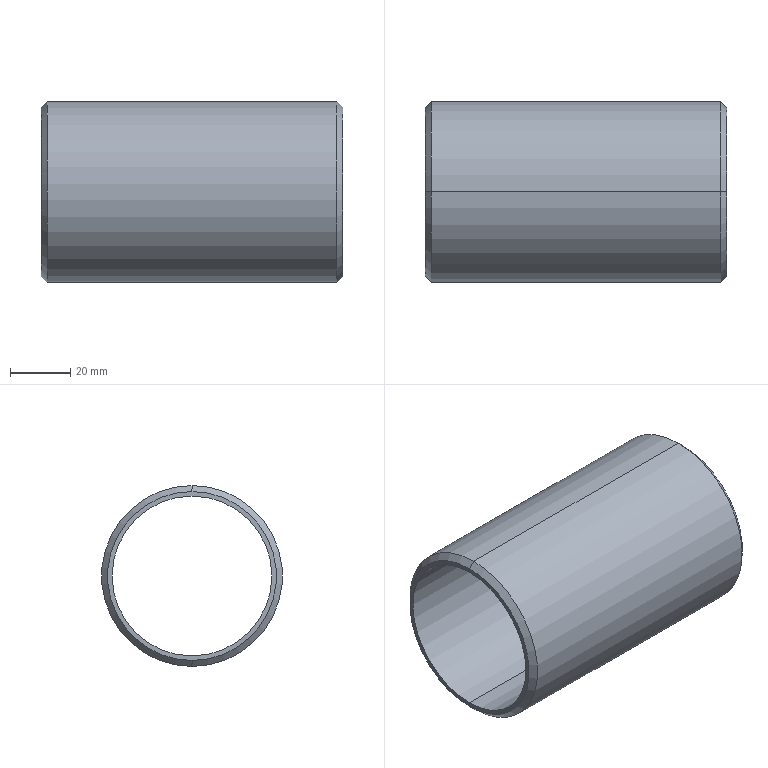Part | SolidWorks | features Chamfer 1, ExtruThin 1 | 1 solid | 10 faces | box 100 x 60 x 60 mm | volume 61388 mm3 | cone 4 | cylinder 4 | plane 2 | commonest cylinder face diameters 53 x2 60 x2
STEP:
#1=CARTESIAN_POINT('',(0.,0.,28.));
#2=VERTEX_POINT('',#1);
#3=CARTESIAN_POINT('',(0.,0.,-28.));
#4=VERTEX_POINT('',#3);
#5=CARTESIAN_POINT('',(0.,0.,0.));
#6=DIRECTION('',(-1.,0.,0.));
#7=DIRECTION('',(0.,0.,-1.));
#8=AXIS2_PLACEMENT_3D('',#5,#6,#7);
#9=CIRCLE('',#8,28.);
#10=EDGE_CURVE('',#2,#4,#9,.T.);
#11=ORIENTED_EDGE('',*,*,#10,.F.);
#12=CARTESIAN_POINT('',(2.,0.,30.));
#13=VERTEX_POINT('',#12);
#14=CARTESIAN_POINT('',(2.,0.,30.));
#15=DIRECTION('',(0.7071,0.,0.7071));
#16=VECTOR('',#15,1000.);
#17=LINE('',#14,#16);
#18=EDGE_CURVE('',#2,#13,#17,.T.);
#19=ORIENTED_EDGE('',*,*,#18,.T.);
#20=CARTESIAN_POINT('',(2.,0.,-30.));
#21=VERTEX_POINT('',#20);
#22=CARTESIAN_POINT('',(2.,0.,0.));
#23=DIRECTION('',(1.,0.,0.));
#24=DIRECTION('',(0.,0.,-1.));
#25=AXIS2_PLACEMENT_3D('',#22,#23,#24);
#26=CIRCLE('',#25,30.);
#27=EDGE_CURVE('',#21,#13,#26,.T.);
#28=ORIENTED_EDGE('',*,*,#27,.F.);
#29=CARTESIAN_POINT('',(2.,0.,-30.));
#30=DIRECTION('',(0.7071,0.,-0.7071));
#31=VECTOR('',#30,1000.);
#32=LINE('',#29,#31);
#33=EDGE_CURVE('',#4,#21,#32,.T.);
#34=ORIENTED_EDGE('',*,*,#33,.F.);
#35=EDGE_LOOP('',(#11,#19,#28,#34));
#36=FACE_OUTER_BOUND('',#35,.T.);
#37=CARTESIAN_POINT('',(2.,0.,0.));
#38=DIRECTION('',(1.,0.,0.));
#39=DIRECTION('',(0.,0.,-1.));
#40=AXIS2_PLACEMENT_3D('',#37,#38,#39);
#41=CONICAL_SURFACE('',#40,30.,0.7854);
#42=ADVANCED_FACE('',(#36),#41,.T.);
#43=CARTESIAN_POINT('',(100.,0.,-28.));
#44=VERTEX_POINT('',#43);
#45=CARTESIAN_POINT('',(100.,0.,28.));
#46=VERTEX_POINT('',#45);
#47=CARTESIAN_POINT('',(100.,0.,0.));
#48=DIRECTION('',(1.,0.,0.));
#49=DIRECTION('',(0.,0.,-1.));
#50=AXIS2_PLACEMENT_3D('',#47,#48,#49);
#51=CIRCLE('',#50,28.);
#52=EDGE_CURVE('',#44,#46,#51,.T.);
#53=ORIENTED_EDGE('',*,*,#52,.F.);
#54=CARTESIAN_POINT('',(98.,0.,-30.));
#55=VERTEX_POINT('',#54);
#56=CARTESIAN_POINT('',(100.,0.,-28.));
#57=DIRECTION('',(-0.7071,0.,-0.7071));
#58=VECTOR('',#57,1000.);
#59=LINE('',#56,#58);
#60=EDGE_CURVE('',#44,#55,#59,.T.);
#61=ORIENTED_EDGE('',*,*,#60,.T.);
#62=CARTESIAN_POINT('',(98.,0.,30.));
#63=VERTEX_POINT('',#62);
#64=CARTESIAN_POINT('',(98.,0.,0.));
#65=DIRECTION('',(-1.,0.,0.));
#66=DIRECTION('',(0.,0.,-1.));
#67=AXIS2_PLACEMENT_3D('',#64,#65,#66);
#68=CIRCLE('',#67,30.);
#69=EDGE_CURVE('',#63,#55,#68,.T.);
#70=ORIENTED_EDGE('',*,*,#69,.F.);
#71=CARTESIAN_POINT('',(100.,0.,28.));
#72=DIRECTION('',(-0.7071,0.,0.7071));
#73=VECTOR('',#72,1000.);
#74=LINE('',#71,#73);
#75=EDGE_CURVE('',#46,#63,#74,.T.);
#76=ORIENTED_EDGE('',*,*,#75,.F.);
#77=EDGE_LOOP('',(#53,#61,#70,#76));
#78=FACE_OUTER_BOUND('',#77,.T.);
#79=CARTESIAN_POINT('',(100.,0.,0.));
#80=DIRECTION('',(-1.,0.,0.));
#81=DIRECTION('',(0.,0.,1.));
#82=AXIS2_PLACEMENT_3D('',#79,#80,#81);
#83=CONICAL_SURFACE('',#82,28.,0.7854);
#84=ADVANCED_FACE('',(#78),#83,.T.);
#85=CARTESIAN_POINT('',(100.,0.,26.5));
#86=VERTEX_POINT('',#85);
#87=CARTESIAN_POINT('',(100.,0.,-26.5));
#88=VERTEX_POINT('',#87);
#89=CARTESIAN_POINT('',(100.,0.,0.));
#90=DIRECTION('',(1.,0.,0.));
#91=DIRECTION('',(0.,0.,-1.));
#92=AXIS2_PLACEMENT_3D('',#89,#90,#91);
#93=CIRCLE('',#92,26.5);
#94=EDGE_CURVE('',#86,#88,#93,.T.);
#95=ORIENTED_EDGE('',*,*,#94,.T.);
#96=CARTESIAN_POINT('',(0.,0.,-26.5));
#97=VERTEX_POINT('',#96);
#98=CARTESIAN_POINT('',(100.,0.,-26.5));
#99=DIRECTION('',(-1.,0.,0.));
#100=VECTOR('',#99,1000.);
#101=LINE('',#98,#100);
#102=EDGE_CURVE('',#88,#97,#101,.T.);
#103=ORIENTED_EDGE('',*,*,#102,.T.);
#104=CARTESIAN_POINT('',(0.,0.,26.5));
#105=VERTEX_POINT('',#104);
#106=CARTESIAN_POINT('',(0.,0.,0.));
#107=DIRECTION('',(1.,0.,0.));
#108=DIRECTION('',(0.,0.,-1.));
#109=AXIS2_PLACEMENT_3D('',#106,#107,#108);
#110=CIRCLE('',#109,26.5);
#111=EDGE_CURVE('',#105,#97,#110,.T.);
#112=ORIENTED_EDGE('',*,*,#111,.F.);
#113=CARTESIAN_POINT('',(100.,0.,26.5));
#114=DIRECTION('',(-1.,0.,0.));
#115=VECTOR('',#114,1000.);
#116=LINE('',#113,#115);
#117=EDGE_CURVE('',#86,#105,#116,.T.);
#118=ORIENTED_EDGE('',*,*,#117,.F.);
#119=EDGE_LOOP('',(#95,#103,#112,#118));
#120=FACE_OUTER_BOUND('',#119,.T.);
#121=CARTESIAN_POINT('',(100.,0.,0.));
#122=DIRECTION('',(-1.,0.,0.));
#123=DIRECTION('',(0.,0.,1.));
#124=AXIS2_PLACEMENT_3D('',#121,#122,#123);
#125=CYLINDRICAL_SURFACE('',#124,26.5);
#126=ADVANCED_FACE('',(#120),#125,.F.);
#127=ORIENTED_EDGE('',*,*,#69,.T.);
#128=CARTESIAN_POINT('',(100.,0.,-30.));
#129=DIRECTION('',(-1.,0.,0.));
#130=VECTOR('',#129,1000.);
#131=LINE('',#128,#130);
#132=EDGE_CURVE('',#55,#21,#131,.T.);
#133=ORIENTED_EDGE('',*,*,#132,.T.);
#134=ORIENTED_EDGE('',*,*,#27,.T.);
#135=CARTESIAN_POINT('',(100.,0.,30.));
#136=DIRECTION('',(-1.,0.,0.));
#137=VECTOR('',#136,1000.);
#138=LINE('',#135,#137);
#139=EDGE_CURVE('',#63,#13,#138,.T.);
#140=ORIENTED_EDGE('',*,*,#139,.F.);
#141=EDGE_LOOP('',(#127,#133,#134,#140));
#142=FACE_OUTER_BOUND('',#141,.T.);
#143=CARTESIAN_POINT('',(100.,0.,0.));
#144=DIRECTION('',(-1.,0.,0.));
#145=DIRECTION('',(0.,0.,1.));
#146=AXIS2_PLACEMENT_3D('',#143,#144,#145);
#147=CYLINDRICAL_SURFACE('',#146,30.);
#148=ADVANCED_FACE('',(#142),#147,.T.);
#149=CARTESIAN_POINT('',(100.,0.,0.));
#150=DIRECTION('',(1.,0.,0.));
#151=DIRECTION('',(0.,0.,-1.));
#152=AXIS2_PLACEMENT_3D('',#149,#150,#151);
#153=CIRCLE('',#152,28.);
#154=EDGE_CURVE('',#46,#44,#153,.T.);
#155=ORIENTED_EDGE('',*,*,#154,.T.);
#156=ORIENTED_EDGE('',*,*,#52,.T.);
#157=EDGE_LOOP('',(#155,#156));
#158=FACE_OUTER_BOUND('',#157,.T.);
#159=ORIENTED_EDGE('',*,*,#94,.F.);
#160=CARTESIAN_POINT('',(100.,0.,0.));
#161=DIRECTION('',(1.,0.,0.));
#162=DIRECTION('',(0.,0.,-1.));
#163=AXIS2_PLACEMENT_3D('',#160,#161,#162);
#164=CIRCLE('',#163,26.5);
#165=EDGE_CURVE('',#88,#86,#164,.T.);
#166=ORIENTED_EDGE('',*,*,#165,.F.);
#167=EDGE_LOOP('',(#159,#166));
#168=FACE_BOUND('',#167,.T.);
#169=CARTESIAN_POINT('',(100.,0.,0.));
#170=DIRECTION('',(1.,0.,0.));
#171=DIRECTION('',(0.,0.,-1.));
#172=AXIS2_PLACEMENT_3D('',#169,#170,#171);
#173=PLANE('',#172);
#174=ADVANCED_FACE('',(#158,#168),#173,.T.);
#175=CARTESIAN_POINT('',(0.,0.,0.));
#176=DIRECTION('',(-1.,0.,0.));
#177=DIRECTION('',(0.,0.,-1.));
#178=AXIS2_PLACEMENT_3D('',#175,#176,#177);
#179=CIRCLE('',#178,28.);
#180=EDGE_CURVE('',#4,#2,#179,.T.);
#181=ORIENTED_EDGE('',*,*,#180,.T.);
#182=ORIENTED_EDGE('',*,*,#10,.T.);
#183=EDGE_LOOP('',(#181,#182));
#184=FACE_OUTER_BOUND('',#183,.T.);
#185=ORIENTED_EDGE('',*,*,#111,.T.);
#186=CARTESIAN_POINT('',(0.,0.,0.));
#187=DIRECTION('',(1.,0.,0.));
#188=DIRECTION('',(0.,0.,-1.));
#189=AXIS2_PLACEMENT_3D('',#186,#187,#188);
#190=CIRCLE('',#189,26.5);
#191=EDGE_CURVE('',#97,#105,#190,.T.);
#192=ORIENTED_EDGE('',*,*,#191,.T.);
#193=EDGE_LOOP('',(#185,#192));
#194=FACE_BOUND('',#193,.T.);
#195=CARTESIAN_POINT('',(0.,0.,0.));
#196=DIRECTION('',(1.,0.,0.));
#197=DIRECTION('',(0.,0.,-1.));
#198=AXIS2_PLACEMENT_3D('',#195,#196,#197);
#199=PLANE('',#198);
#200=ADVANCED_FACE('',(#184,#194),#199,.F.);
#201=ORIENTED_EDGE('',*,*,#132,.F.);
#202=CARTESIAN_POINT('',(98.,0.,0.));
#203=DIRECTION('',(-1.,0.,0.));
#204=DIRECTION('',(0.,0.,-1.));
#205=AXIS2_PLACEMENT_3D('',#202,#203,#204);
#206=CIRCLE('',#205,30.);
#207=EDGE_CURVE('',#55,#63,#206,.T.);
#208=ORIENTED_EDGE('',*,*,#207,.T.);
#209=ORIENTED_EDGE('',*,*,#139,.T.);
#210=CARTESIAN_POINT('',(2.,0.,0.));
#211=DIRECTION('',(1.,0.,0.));
#212=DIRECTION('',(0.,0.,-1.));
#213=AXIS2_PLACEMENT_3D('',#210,#211,#212);
#214=CIRCLE('',#213,30.);
#215=EDGE_CURVE('',#13,#21,#214,.T.);
#216=ORIENTED_EDGE('',*,*,#215,.T.);
#217=EDGE_LOOP('',(#201,#208,#209,#216));
#218=FACE_OUTER_BOUND('',#217,.T.);
#219=CARTESIAN_POINT('',(100.,0.,0.));
#220=DIRECTION('',(-1.,0.,0.));
#221=DIRECTION('',(0.,0.,1.));
#222=AXIS2_PLACEMENT_3D('',#219,#220,#221);
#223=CYLINDRICAL_SURFACE('',#222,30.);
#224=ADVANCED_FACE('',(#218),#223,.T.);
#225=ORIENTED_EDGE('',*,*,#102,.F.);
#226=ORIENTED_EDGE('',*,*,#165,.T.);
#227=ORIENTED_EDGE('',*,*,#117,.T.);
#228=ORIENTED_EDGE('',*,*,#191,.F.);
#229=EDGE_LOOP('',(#225,#226,#227,#228));
#230=FACE_OUTER_BOUND('',#229,.T.);
#231=CARTESIAN_POINT('',(100.,0.,0.));
#232=DIRECTION('',(-1.,0.,0.));
#233=DIRECTION('',(0.,0.,1.));
#234=AXIS2_PLACEMENT_3D('',#231,#232,#233);
#235=CYLINDRICAL_SURFACE('',#234,26.5);
#236=ADVANCED_FACE('',(#230),#235,.F.);
#237=ORIENTED_EDGE('',*,*,#60,.F.);
#238=ORIENTED_EDGE('',*,*,#154,.F.);
#239=ORIENTED_EDGE('',*,*,#75,.T.);
#240=ORIENTED_EDGE('',*,*,#207,.F.);
#241=EDGE_LOOP('',(#237,#238,#239,#240));
#242=FACE_OUTER_BOUND('',#241,.T.);
#243=CARTESIAN_POINT('',(100.,0.,0.));
#244=DIRECTION('',(-1.,0.,0.));
#245=DIRECTION('',(0.,0.,1.));
#246=AXIS2_PLACEMENT_3D('',#243,#244,#245);
#247=CONICAL_SURFACE('',#246,28.,0.7854);
#248=ADVANCED_FACE('',(#242),#247,.T.);
#249=ORIENTED_EDGE('',*,*,#18,.F.);
#250=ORIENTED_EDGE('',*,*,#180,.F.);
#251=ORIENTED_EDGE('',*,*,#33,.T.);
#252=ORIENTED_EDGE('',*,*,#215,.F.);
#253=EDGE_LOOP('',(#249,#250,#251,#252));
#254=FACE_OUTER_BOUND('',#253,.T.);
#255=CARTESIAN_POINT('',(2.,0.,0.));
#256=DIRECTION('',(1.,0.,0.));
#257=DIRECTION('',(0.,0.,-1.));
#258=AXIS2_PLACEMENT_3D('',#255,#256,#257);
#259=CONICAL_SURFACE('',#258,30.,0.7854);
#260=ADVANCED_FACE('',(#254),#259,.T.);
#261=CLOSED_SHELL('',(#42,#84,#126,#148,#174,#200,#224,#236,#248,#260));
#262=MANIFOLD_SOLID_BREP('',#261);
#263=CARTESIAN_POINT('',(0.,0.,0.));
#264=DIRECTION('',(0.,0.,1.));
#265=DIRECTION('',(1.,0.,0.));
#266=AXIS2_PLACEMENT_3D('',#263,#264,#265);
#267=(LENGTH_UNIT()NAMED_UNIT(*)SI_UNIT(.MILLI.,.METRE.));
#268=UNCERTAINTY_MEASURE_WITH_UNIT(LENGTH_MEASURE(0.00001),#267,'','');
#269=(NAMED_UNIT(*)PLANE_ANGLE_UNIT()SI_UNIT($,.RADIAN.));
#270=(NAMED_UNIT(*)SI_UNIT($,.STERADIAN.)SOLID_ANGLE_UNIT());
#271=(GEOMETRIC_REPRESENTATION_CONTEXT(3)GLOBAL_UNCERTAINTY_ASSIGNED_CONTEXT((#268))GLOBAL_UNIT_ASSIGNED_CONTEXT((#267,#269,#270))REPRESENTATION_CONTEXT('',''));
#272=ADVANCED_BREP_SHAPE_REPRESENTATION('',(#262,#266),#271);